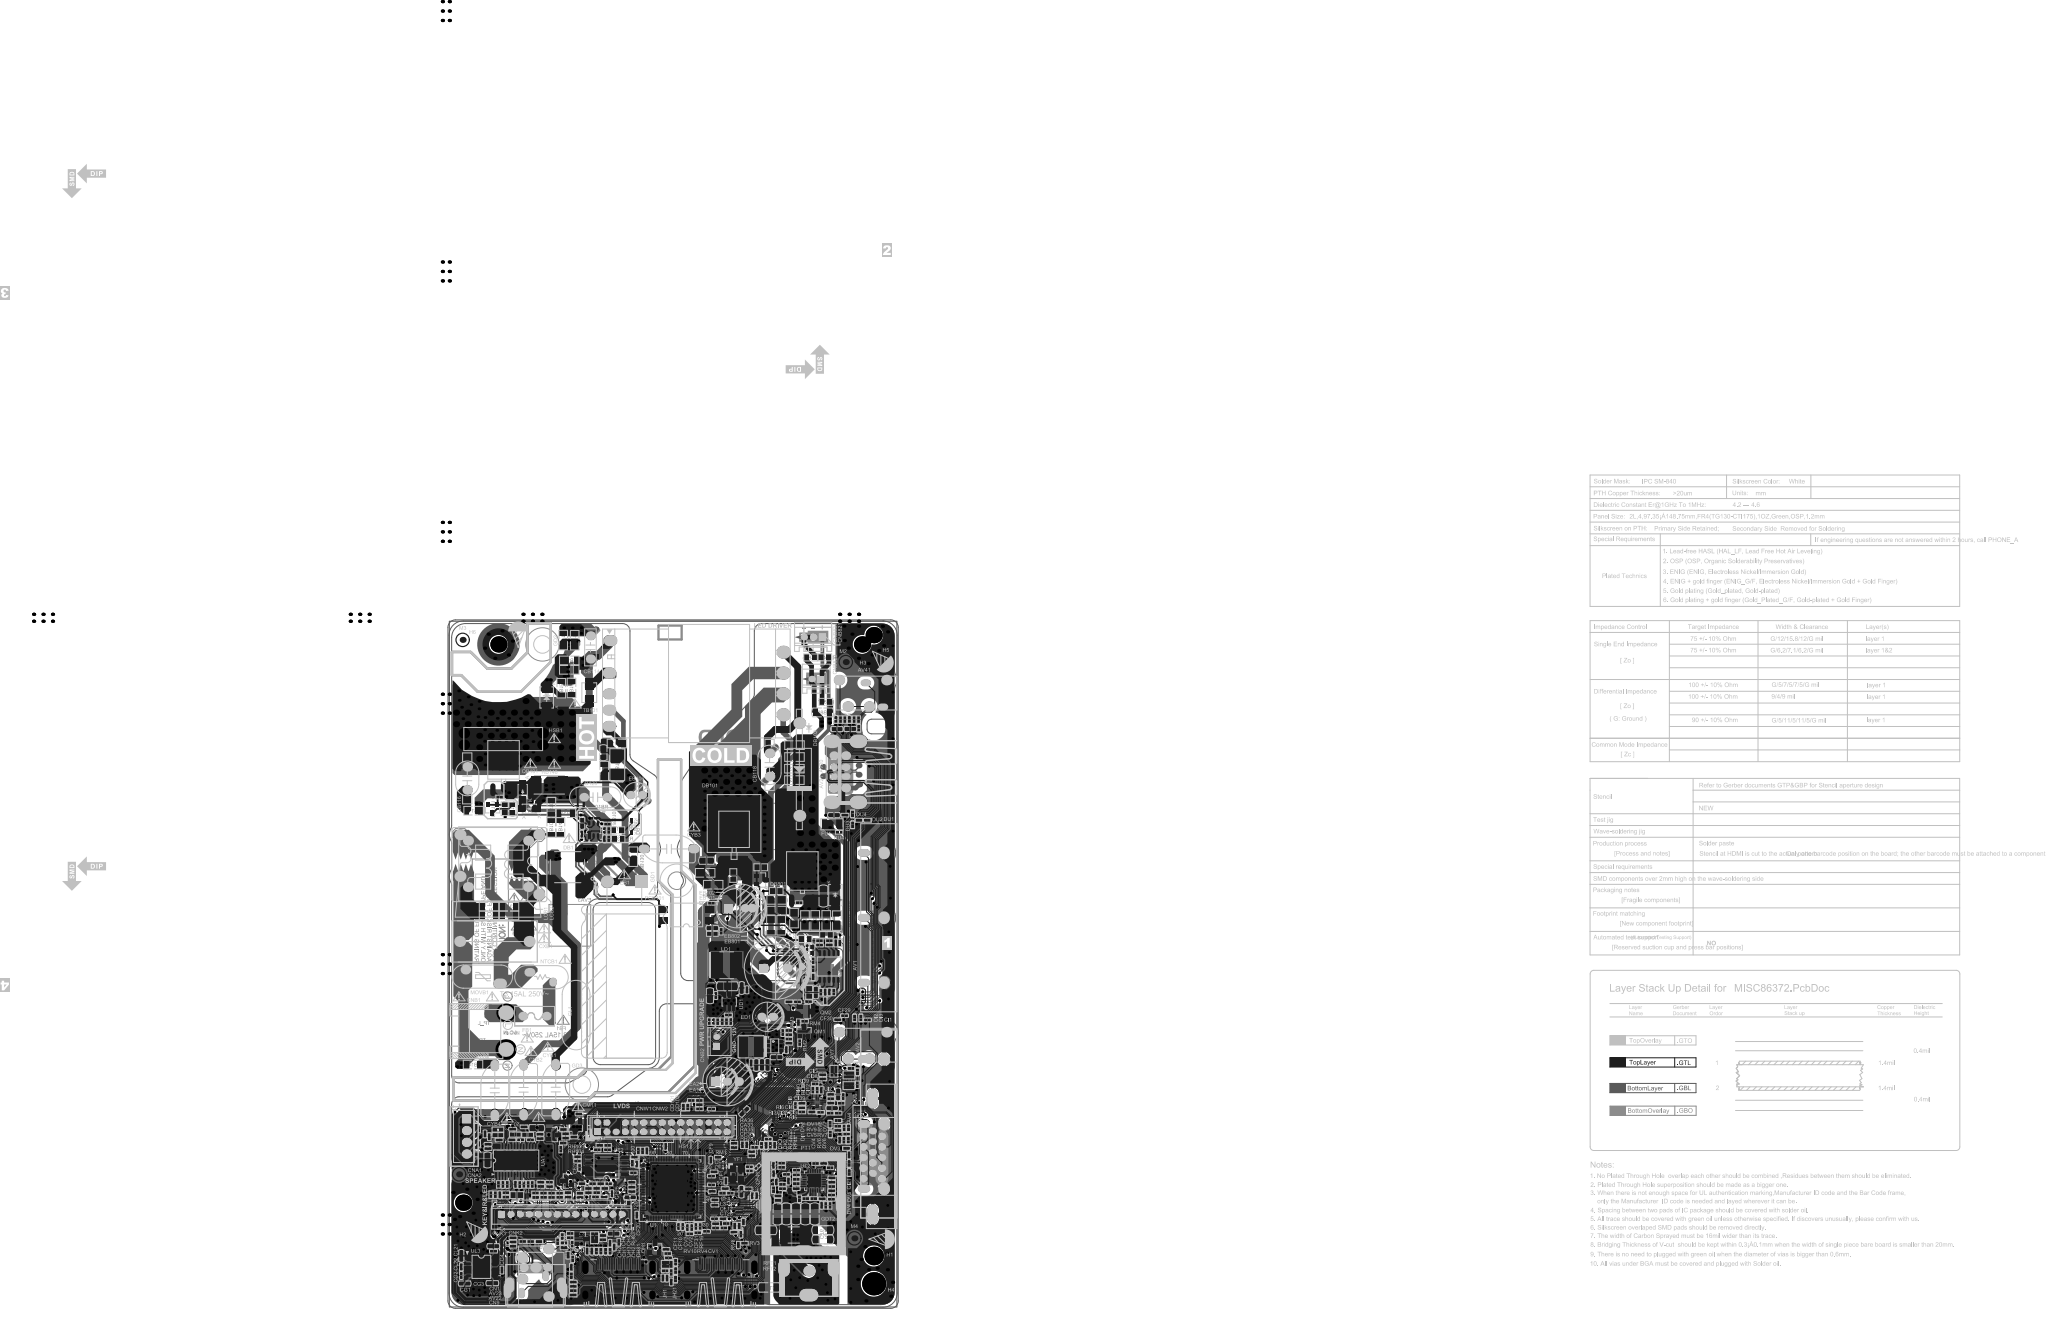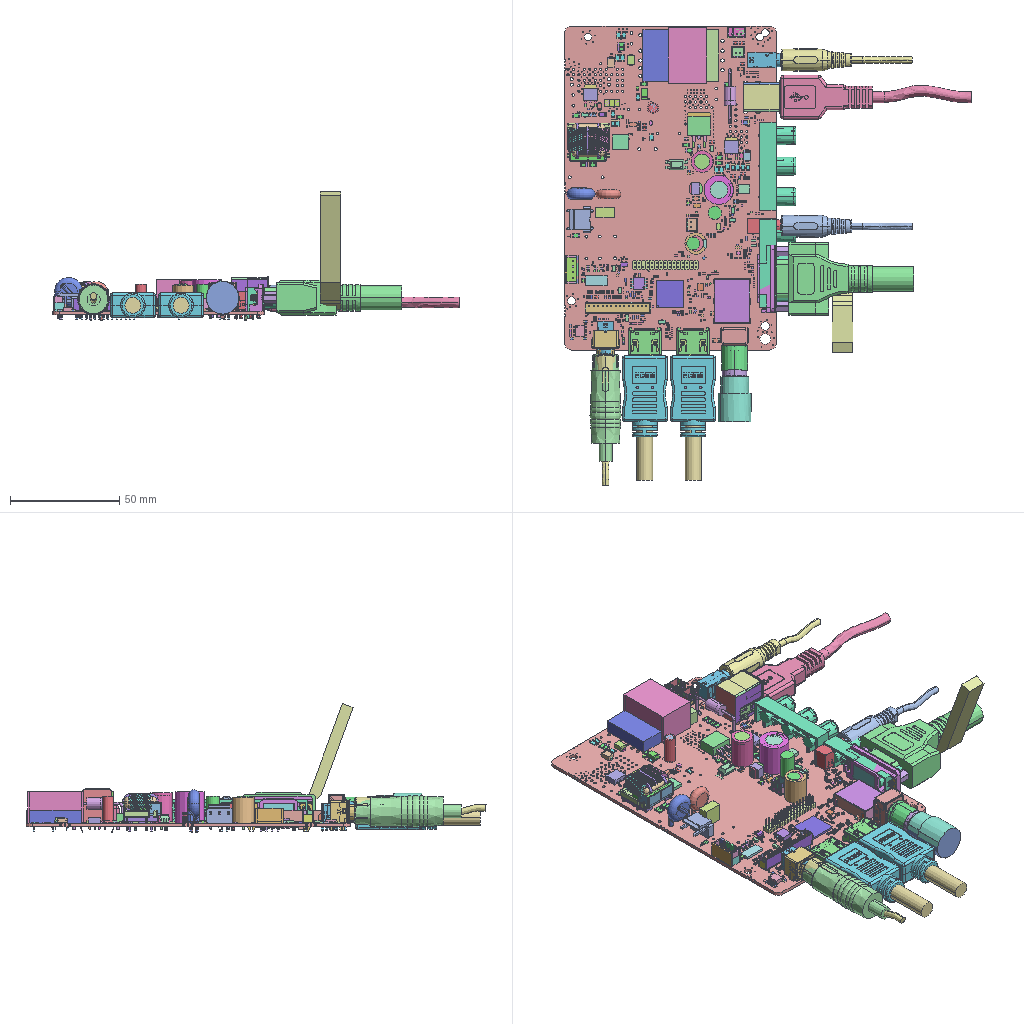Circuit board layout | Altium Designer | box 185.9 x 210.3 x 58.9 mm
Layer stack:
# Altium Designer layer stack of  (unit mm; dielectric type: 0 none, 1 core, 2 prepreg, 3 surface material)
index,name,kind,layer,copper_thickness_mm,dielectric_type,dielectric_thickness_mm,dielectric_material,dielectric_constant
0,TopPaste,other,,,,,,
1,TopOverlay,other,,,,,,
2,TopSolder,dielectric,,,3,0.0102,Solder Resist,3.5
3,TopLayer,copper,TopLayer,0.0356,,,,
4,Dielectric1,dielectric,,,1,1.5,FR-4,4.8
5,BottomLayer,copper,BottomLayer,0.0356,,,,
6,BottomSolder,dielectric,,,3,0.0102,Solder Resist,3.5
7,BottomOverlay,other,,,,,,
8,BottomPaste,other,,,,,,
# drill layer pairs: low layer,high layer
drill_pair,TopLayer,BottomLayer
Part placement, first 359 of 579 lines:
Designator,Comment,Layer,Footprint,Center-X(mm),Center-Y(mm),Rotation
DI6,NC/NC/AVLC18S02003,TopLayer,DIODE-S0402,-71.831,13.818,180
CO13,NC/1000pF-0402-X7R-¡À10%-50V,TopLayer,C0402,-71.831,12.802,180
CO12,NC/Ceramic capacitor,CAP MC,6.3V,0.47uF,¡À10%,X5R,0402,SMD,TP,TopLayer,C0402,-70.968,11.176,270
Manufacture_Info,Manufacture_Info,TopLayer,Manufacture_Info,-31.626,103.746,180
CT47,NC/Ceramic capacitor,CAP MC,1KV,4700pF,¡À10%,X7R,1206,SMD,TP,TopLayer,C1206,-28.27,16.56,360
CK3,Ceramic capacitor,CAP MC,50V,0.01uF,¡À10%,X7R,0402,SMD,TP,TopLayer,C0402,-63.17,23.749,180
RK13,33Kohm-0402-¡À5%-1/16W,TopLayer,R0402,-65.678,26.594,180
UF2,SPI FLASH chip,IC SPI FLASH,4MB,32Mb,SOIC8,SMD,W25Q32JVSSIQ,Winbond,TopLayer,SOIC8,-62.687,30.42,180
DV1,NC/AVLC18S02003,TopLayer,DIODE-S0402,-12.733,40.234,360
RT1,Ferrite bead,BEAD,300ohm,0402,800mA,SMD,TP,FCM1005KF-301T08,TopLayer,R0402,-35.941,24.566,180
RF9,NC/4K7ohm-0402-¡À5%-1/16W,TopLayer,R0402,-44.374,44.564,360
RF8,NC/4K7ohm-0402-¡À5%-1/16W,TopLayer,R0402,-42.647,44.564,180
EA2,NC/Aluminium electrolytic capacitor,CAP AL,16V,220uF,¡À20%,LD,KF,P,2.5mm,6.3¡Á11,DIP,TP,CapXon,TopLayer,EC(6.3*11)-V-2.5,-37.908,48.199,360
CNA2,NC/4PIN-2.54-D-H-G-latched-B,TopLayer,SIP4/2.5D-2,-92.877,36.793,270
CL4,NC/1uF-0402-X5R-¡À20%-6.3V,TopLayer,C0402,-26.01,26.988,90
CL3,10uF-0603-X5R-¡À20%-6.3V,TopLayer,C0603,-33.55,24.889,270
CI1,NC/10pF-0402-NPO-¡À5%-50V,TopLayer,C0402,-6.35,61.951,180
UART_TX,DM0,BottomLayer,TP,-25.349,49.047,90
RPI1,Resistor array,RES ARRAY,1/16W,4¡Á10Kohm,¡À5%,0402,SMD,TopLayer,RA0402,-13.589,50.876,180
DV8,NC/AVLC18S02003,TopLayer,DIODE-S0402,-9.881,51.486,180
DV9,NC/AVLC18S02003,TopLayer,DIODE-S0402,-8.509,50.749,270
RPV1,NC/Resistor array,RES ARRAY,1/16W,4¡Á10Kohm,¡À5%,0402,SMD,TopLayer,RA0402,-10.342,50.082,270
RF43,4K7ohm-0402-¡À5%-1/16W,TopLayer,R0402,-27.305,34.9,270
RF44,4K7ohm-0402-¡À5%-1/16W,TopLayer,R0402,-26.391,34.9,270
RU1,NC/0ohm-0402-PCB,TopLayer,R0402SC,-35.149,34.413,360
RU2,NC/0ohm-0402-PCB,TopLayer,R0402SC,-35.149,35.327,360
RU5,NC/0ohm-0402-PCB,TopLayer,R0402SC,-33.336,34.99,90
RI5,NC/0ohm-0402-¡À5%-1/16W,TopLayer,R0402,-16.471,41.992,180
CI3,NC/0.1uF-0402-X5R-¡À20%-16V,TopLayer,C0402,-16.471,41.993,360
CI4,NC/0.1uF-0402-X5R-¡À20%-16V,TopLayer,C0402,-20.496,42.996,360
CI6,0.1uF-0402-X5R-¡À20%-16V,TopLayer,C0402,-16.007,50.126,360
CV4,NC/30pF-0402-NPO-¡À5%-50V,TopLayer,C0402,-12.37,35.992,90
CV5,NC/30pF-0402-NPO-¡À5%-50V,TopLayer,C0402,-12.739,38.093,180
DV2,NC/AVLC18S02003,TopLayer,DIODE-S0402,-14.427,39.478,270
DV3,NC/AVLC18S02003,TopLayer,DIODE-S0402,-10.897,34.239,360
DV4,NC/AVLC18S02003,TopLayer,DIODE-S0402,-10.287,28.981,90
DV5,NC/AVLC18S02003,TopLayer,DIODE-S0402,-10.312,30.937,90
DV6,NC/AVLC18S02003,TopLayer,DIODE-S0402,-10.49,35.992,90
DV7,NC/AVLC18S02003,TopLayer,DIODE-S0402,-10.431,38.633,90
RF10,NC/100ohm-0402-¡À5%-1/16W,TopLayer,R0402,-42.639,43.649,360
RF11,NC/100ohm-0402-¡À5%-1/16W,TopLayer,R0402,-42.621,42.739,360
RM1,10Kohm-0402-¡À5%-1/16W,TopLayer,R0402,-38.608,32.309,180
RV6,NC/10Kohm-0402-¡À5%-1/16W,TopLayer,R0402,-11.43,35.992,90
RV7,NC/100ohm-0402-¡À5%-1/16W,TopLayer,R0402,-10.846,37.313,180
RV8,NC/10Kohm-0402-¡À5%-1/16W,TopLayer,R0402,-11.396,38.633,90
RV9,NC/100ohm-0402-¡À5%-1/16W,TopLayer,R0402,-12.751,39.011,180
RI6,NC/0ohm-0402-¡À5%-1/16W,TopLayer,R0402,-20.496,42.996,180
CA33,Ceramic capacitor,CAP MC,6.3V,0.47uF,¡À10%,X5R,0402,SMD,TP,TopLayer,C0402,-31.323,33.528,360
CI8,0.1uF-0402-X5R-¡À20%-16V,TopLayer,C0402,-21.895,43.51,90
CI9,NC/NC/10uF-0603-X5R-¡À20%-6.3V,TopLayer,C0603,-12.675,45.872,270
CI12,NC/Ceramic capacitor,CAP MC,6.3V,0.47uF,¡À10%,X5R,0402,SMD,TP,TopLayer,C0402,-16.298,46.805,90
CI35,NC/1000pF-0402-X7R-¡À10%-50V,TopLayer,C0402,-18.335,42.088,360
CI36,NC/0.1uF-0402-X5R-¡À20%-16V,TopLayer,C0402,-11.582,45.415,270
CI37,NC/Ceramic capacitor,CAP MC,6.3V,0.47uF,¡À10%,X5R,0402,SMD,TP,TopLayer,C0402,-14.275,45.868,360
CI38,NC/Ceramic capacitor,CAP MC,6.3V,0.47uF,¡À10%,X5R,0402,SMD,TP,TopLayer,C0402,-16.002,49.2,360
CI39,NC/Ceramic capacitor,CAP MC,6.3V,0.47uF,¡À10%,X5R,0402,SMD,TP,TopLayer,C0402,-20.502,43.94,180
CI40,NC/10uF-0603-X5R-¡À20%-6.3V,TopLayer,C0603,-13.97,42.901,180
CI41,NC/0.1uF-0402-X5R-¡À20%-16V,TopLayer,C0402,-14.275,43.993,180
RA35,47Kohm-0402-¡À5%-1/16W,TopLayer,R0402,-31.318,32.614,180
RA36,10Kohm-0402-¡À5%-1/16W,TopLayer,R0402,-30.709,34.442,360
RI3,NC/1Kohm-0402-¡À5%-1/16W,TopLayer,R0402,-20.498,42.088,360
RI4,0ohm-0402-¡À5%-1/16W,TopLayer,R0402,-8.534,47.955,90
RI37,NC/200Kohm-0402-¡À5%-1/16W,TopLayer,R0402,-14.275,44.929,360
RI38,NC/200Kohm-0402-¡À5%-1/16W,TopLayer,R0402,-17.212,46.804,90
RI39,NC/200Kohm-0402-¡À5%-1/16W,TopLayer,R0402,-17.653,48.133,180
RI40,NC/200Kohm-0402-¡À5%-1/16W,TopLayer,R0402,-18.127,46.804,90
RI42,NC/1Kohm-0402-¡À5%-1/16W,TopLayer,R0402,-12.675,41.834,360
RI43,NC/1Kohm-0402-¡À5%-1/16W,TopLayer,R0402,-12.04,43.967,360
RI48,NC/100ohm-0402-¡À5%-1/16W,TopLayer,R0402,-14.402,41.834,360
UI2,NC/AZAW2213F,TopLayer,QFN10/0.4,-17.206,44.208,270
CI21,NC/NC/10pF-0402-NPO-¡À5%-50V,TopLayer,C0402,-10.312,32.817,270
RU3,NC/0ohm-0402-PCB,TopLayer,R0402SC,-32.423,34.976,90
RA5,NC/?,TopLayer,GND,-32.31,21.262,180
RA4,NC/?,TopLayer,GND,-33.96,20.498,180
L6,0ohm-0402-¡À5%-1/16W,TopLayer,R0402,-14.427,30.041,180
CF40,Ceramic capacitor,CAP MC,50V,0.01uF,¡À10%,X7R,0402,SMD,TP,TopLayer,C0402,-30.099,30.201,225
UT2,Silicon RF tuner,IC Si Tuner,QFN24,SMD,R842,Rafael,TopLayer,QFN24/0.5-3,-17.882,27.254,90
RT8,100ohm-0402-¡À5%-1/16W,TopLayer,R0402,-17.551,30.963,180
RT6,1K8ohm-0402-¡À5%-1/16W,TopLayer,R0402,-14.05,25.988,180
RT5,0ohm-0402-¡À5%-1/16W,TopLayer,R0402,-24.867,31.039,180
RT4,0ohm-0402-¡À5%-1/16W,TopLayer,R0402,-24.867,30.124,180
RT3,22ohm-0402-¡À5%-1/16W,TopLayer,R0402,-14.431,21.924,90
RT2,22ohm-0402-¡À5%-1/16W,TopLayer,R0402,-15.345,21.924,90
LT10,NC/SDCL1005CR18JTDF(180nH-0402¡À5%-C),TopLayer,L0402,-24.707,26.474,180
LT9,Multilayer inductor,HF Inductor,270nH,¡À5%,0402,SMD,SDCL1005CR27JTDF,Sunlord,TopLayer,L0402,-21.717,27.564,180
LT8,Multilayer inductor,,HF Inductor,39nH,¡À5%,0402,SMD,SDCL1005C39NJTDF,Sunlord,TopLayer,L0402,-21.717,26.599,360
LT6,SDCL1005CR18JTDF(180nH-0402¡À5%-C),TopLayer,L0402,-17.933,23.368,180
LT5,GZ1005U102CTF(1000ohm-300mA),TopLayer,L0402,-19.66,23.368,180
LT4,GZ1005U102CTF(1000ohm-300mA),TopLayer,L0402,-21.031,23.343,270
LT3,NC/SDCL1005CR18JTDF(180nH-0402¡À5%-C),TopLayer,L0402,-26.619,25.299,90
LT2,NC/SDCL1005CR27JTDF(Sunlord),TopLayer,L0402,-25.654,23.012,180
CT27,0.1uF-0402-X5R-¡À20%-16V,TopLayer,C0402,-15.799,30.963,180
CT25,0.1uF-0402-X5R-¡À20%-16V,TopLayer,C0402,-14.021,27.864,360
CT24,6800pF-0402-X7R-¡À10%-50V,TopLayer,C0402,-14.072,25.07,180
CT23,330pF-0402-NPO-¡À5%-50V,TopLayer,C0402,-14.05,26.903,180
CT22,0.1uF-0402-X5R-¡À20%-16V,TopLayer,C0402,-14.117,24.154,360
CT21,0.1uF-0402-X5R-¡À20%-16V,TopLayer,C0402,-21.666,29.515,360
CT20,0.022uF-0402-X7R-¡À10%-16V,TopLayer,C0402,-23.829,28.6,180
CT19,0.022uF-0402-X7R-¡À10%-16V,TopLayer,C0402,-21.692,28.504,360
CT18,NC/1000pF-0402-X7R-¡À10%-50V,TopLayer,C0402,-23.393,27.178,270
CT17,0.1uF-0402-X5R-¡À20%-16V,TopLayer,C0402,-21.717,25.532,360
CT16,0.047uF-0402-X7R-¡À10%-16V,TopLayer,C0402,-16.129,23.343,360
CT15,0ohm-0402-¡À5%-1/16W,TopLayer,C0402,-24.706,25.535,360
CT14,NC/220pF-0402-NPO-¡À5%-50V,TopLayer,C0402,-25.654,23.952,180
CT10,NC/30pF-0402-NPO-¡À5%-50V,TopLayer,C0402,-26.645,30.582,90
CT8,NC/30pF-0402-NPO-¡À5%-50V,TopLayer,C0402,-26.619,28.727,90
CT7,Ceramic capacitor,CAP MC,50V,22pF,¡À5%,NPO,0402,SMD,TP,TopLayer,C0402,-14.117,23.239,180
CT6,Ceramic capacitor,CAP MC,50V,22pF,¡À5%,NPO,0402,SMD,TP,TopLayer,C0402,-16.259,21.95,90
DT1,KAV99,TopLayer,SO-23,-23.139,24.105,180
CF1,Ceramic capacitor,CAP MC,50V,18pF,¡À5%,NPO,0402,SMD,TP,TopLayer,C0402,-36.906,27.178,270
CF4,Ceramic capacitor,CAP MC,50V,18pF,¡À5%,NPO,0402,SMD,TP,TopLayer,C0402,-37.059,25.552,180
CF9,0.1uF-0402-X5R-¡À20%-16V,TopLayer,C0402,-40.174,31.689,270
CF10,0.1uF-0402-X5R-¡À20%-16V,TopLayer,C0402,-46.226,17.375,90
CF11,0.1uF-0402-X5R-¡À20%-16V,TopLayer,C0402,-47.14,17.375,270
CF12,0.1uF-0402-X5R-¡À20%-16V,TopLayer,C0402,-39.294,23.114,180
CF13,0.1uF-0402-X5R-¡À20%-16V,TopLayer,C0402,-39.115,17.975,180
CF14,0.1uF-0402-X5R-¡À20%-16V,TopLayer,C0402,-39.876,24.942,180
CF17,0.1uF-0402-X5R-¡À20%-16V,TopLayer,C0402,-40.005,26.34,180
CF19,0.1uF-0402-X5R-¡À20%-16V,TopLayer,C0402,-39.446,29.159,360
CF24,Ceramic capacitor,CAP MC,6.3V,2.2uF,¡À20%,X5R,0402,SMD,TP,TopLayer,C0402,-40.03,28.245,360
CF26,0.047uF-0402-X7R-¡À10%-16V,TopLayer,C0402,-39.116,17.044,360
CF27,NC/0.1uF-0402-X5R-¡À20%-16V,TopLayer,C0402,-37.484,19.043,180
CF28,1uF-0402-X5R-¡À20%-6.3V,TopLayer,C0402,-39.359,19.039,360
CF31,0.047uF-0402-X7R-¡À10%-16V,TopLayer,C0402,-43.383,17.373,270
CF38,NC/30pF-0402-NPO-¡À5%-50V,TopLayer,C0402,-31.833,30.251,360
CT11,0.1uF-0402-X5R-¡À20%-16V,TopLayer,C0402,-30.277,24.003,90
CT12,0.1uF-0402-X5R-¡À20%-16V,TopLayer,C0402,-31.191,24.003,90
CT26,0.022uF-0402-X7R-¡À10%-16V,TopLayer,C0402,-39.294,21.971,180
CV1,0.047uF-0402-X7R-¡À10%-16V,TopLayer,C0402,-41.097,16.307,180
CV2,0.047uF-0402-X7R-¡À10%-16V,TopLayer,C0402,-44.298,17.12,90
CV3,0.047uF-0402-X7R-¡À10%-16V,TopLayer,C0402,-45.215,17.12,90
L3,0ohm-0402-¡À5%-1/16W,TopLayer,L0402,-37.643,24.563,180
LF6,NC/?,TopLayer,GND,-37.998,19.66,180
RF12,68ohm-0402-¡À5%-1/16W,TopLayer,R0402,-37.338,17.043,360
RF16,68ohm-0402-¡À5%-1/16W,TopLayer,R0402,-42.469,17.374,90
RF24,1Kohm-0402-¡À5%-1/16W,TopLayer,R0402,-31.814,29.352,180
RV4,33ohm-0402-¡À5%-1/16W,TopLayer,R0402,-42.977,16.002,180
RV10,33ohm-0402-¡À5%-1/16W,TopLayer,R0402,-44.704,15.773,180
YF1,Passive crystal,SPXO,24MHz,¡À10ppm,12pF,SMD3225,SMD,2.3.3.240001234,MDH,TopLayer,XTAL-S-3,-34.519,28.677,270
DK2,NC/AVLC18S02003,TopLayer,DIODE-S0402,-28.245,34.9,270
DK3,NC/AVLC18S02003,TopLayer,DIODE-S0402,-29.21,34.9,270
CT1,NC/0.1uF-0402-X5R-¡À20%-16V,TopLayer,C0402,-27.737,36.22,180
RT7,10Kohm-0402-¡À5%-1/16W,TopLayer,R0402,-32.055,25.476,360
RK6,510ohm-0402-¡À1%-1/16W,TopLayer,R0402,-78.008,24.595,360
GDT2,NC/Gas discharge tube,GDT,700V,2000A,TP,4.5*3.2mm,SMD,4532-091-LF,Brightking,TopLayer,SMD4532-1-C1206,-16.002,15.57,270
GDT1,NC/Gas discharge tube,GDT,700V,2000A,TP,4.5*3.2mm,SMD,4532-091-LF,Brightking,TopLayer,SMD4532-1,-22.25,15.57,360
CT46,Thick-film resistor,RES,1/4W,0ohm,¡À5%,1206,SMD,TopLayer,C1206,-15.977,14.554,180
CT45,Thick-film resistor,RES,1/4W,0ohm,¡À5%,1206,SMD,TopLayer,C1206,-15.977,16.586,180
CT44,Thick-film resistor,RES,1/4W,0ohm,¡À5%,1206,SMD,TopLayer,C1206,-17.729,20.091,270
CT43,Thick-film resistor,RES,1/4W,0ohm,¡À5%,1206,SMD,TopLayer,C1206,-19.761,20.091,270
CT42,Thick-film resistor,RES,1/4W,0ohm,¡À5%,1206,SMD,TopLayer,C1206,-21.768,20.091,270
CT41,Thick-film resistor,RES,1/4W,0ohm,¡À5%,1206,SMD,TopLayer,C1206,-25.756,20.066,270
CT13,Ceramic capacitor,CAP MC,1KV,470pF,¡À5%,NPO,1206,SMD,TP,TopLayer,C1206,-23.851,20.091,90
RO12,NC/510ohm-0402-¡À1%-1/16W,TopLayer,R0402,-69.977,10.363,270
UA1,Audio amplifier,IC Audio AMP,Class D,2¡Á10W@13.0V@8ohm,HTSSOP-28,SMD,RDA3118E28B,RDA,TopLayer,SSOP28/0.65-5,-82.197,31.611,90
QM12,Field-effect transistor,PMOS,-4.3A,-30V,0.048ohm@ID=-3A@VGS=-4.5V,SOT-23-3L,NCE3407AY,NCEPOWER,TopLayer,SOT-23-1,-69.421,38.982,360
RA9,NC/47Kohm-0402-¡À5%-1/16W,TopLayer,R0402,-84.397,23.724,180
VCC_PANEL,TEST,BottomLayer,TP,-67.742,39.878,270
UART_RX,DM0,BottomLayer,TP,-27.686,49.276,90
TXD,,BottomLayer,TP,-62.56,22.631,180
RU4,0ohm-0402-¡À5%-1/16W,TopLayer,R0402,-12.464,102.457,180
RO22,75ohm-0402-¡À5%-1/16W,TopLayer,R0402,-55.804,33.68,270
RO21,Thick-film resistor,RES,1/16W,150ohm,¡À1%,0402,SMD,TopLayer,R0402,-54.89,33.674,270
RM15,NC/4K7ohm-0402-¡À5%-1/16W,TopLayer,R0402,-71.501,37.363,180
RM14,47Kohm-0402-¡À5%-1/16W,TopLayer,R0402,-71.501,36.452,360
RM12,10Kohm-0402-¡À5%-1/16W,TopLayer,R0402,-72.542,34.061,270
RK15,10Kohm-0402-¡À5%-1/16W,TopLayer,R0402,-66.573,24.648,360
RK14,510ohm-0402-¡À1%-1/16W,TopLayer,R0402,-64.795,24.666,360
RK12,4K7ohm-0402-¡À1%-1/16W,TopLayer,R0402,-76.246,23.658,360
RK11,2K2ohm-0402-¡À1%-1/16W,TopLayer,R0402,-74.534,23.641,360
RK10,1Kohm-0402-¡À5%-1/16W,TopLayer,R0402,-68.395,24.544,180
RK9,1K2ohm-0402-¡À1%-1/16W,TopLayer,R0402,-74.535,24.567,360
RK8,1Kohm-0402-¡À1%-1/16W,TopLayer,R0402,-72.791,24.559,360
RK7,680ohm-0402-¡À1%-1/16W,TopLayer,R0402,-72.782,23.663,360
RK5,22ohm-0402-¡À5%-1/16W,TopLayer,R0402,-70.993,24.669,360
RK4,1Kohm-0402-¡À5%-1/16W,TopLayer,R0402,-64.808,25.585,180
QM11,General transistor,Dynatron,NPN,0.2A,40V,30-300,SOT-23,MMBT3904(f¡Ý350MHz),BLUE ROCKET,TopLayer,SOT-23,-74.117,37.211,90
QK1,General transistor,Dynatron,NPN,0.2A,40V,30-300,SOT-23,MMBT3904(f¡Ý350MHz),BLUE ROCKET,TopLayer,SOT-23,-71.171,27.178,270
HS1,NC/Heatsink,6-series aluminium alloy,14.0¡Á14.0¡Á6.0mm,natural,XXWJ,TopLayer,HS(14*14*6),-582.797,-376.375,0
FU1,NC/NSMD110(1206-1.1A),TopLayer,FUSE1.1A-S,-13.994,104.165,180
DK1,NC/AVLC18S02003,TopLayer,DIODE-S0402,-78.01,23.648,360
CO31,NC/NC/33pF-0402-NPO-¡À5%-50V,TopLayer,C0402,-53.975,33.681,90
CO11,NC/1000pF-0402-X7R-¡À10%-50V,TopLayer,C0402,-70.257,8.56,90
CM12,0.022uF-0402-X7R-¡À10%-16V,TopLayer,C0402,-69.694,36.68,180
CM11,NC/0.1uF-0402-X5R-¡À20%-16V,TopLayer,C0402,-68.595,41.652,180
CL21,10uF-0603-X5R-¡À20%-6.3V,TopLayer,C0603,-94.018,11.032,90
CK5,NC/0.1uF-0402-X5R-¡À20%-16V,TopLayer,C0402,-65.056,23.752,360
CK4,NC/0.1uF-0402-X5R-¡À20%-16V,TopLayer,C0402,-68.37,23.63,180
+1.8V_DDR,TEST,BottomLayer,TP,-59.817,23.216,90
UL3,LDO regulator,IC LDO,1A,3.3V,12V,ESOP-8,SMD,LC1118CS8TR1833,Leadchip,TopLayer,SOP8/1.27-3,-89.689,8.66,360
RO33,NC/0ohm-0402-¡À5%-1/16W,TopLayer,R0402,-82.855,13.106,360
RO4,NC/0ohm-0402-¡À5%-1/16W,TopLayer,R0402,-79.045,14.118,180
RO3,NC/0ohm-0402-¡À5%-1/16W,TopLayer,R0402,-80.762,14.129,360
RO2,NC/0ohm-0402-¡À5%-1/16W,TopLayer,R0402,-73.228,14.072,90
DI9,NC/NC/SFI0402-240E-2R5PP-LF,TopLayer,DIODE-S0402,-77.241,14.101,180
CO33,330pF-0402-NPO-¡À5%-50V,TopLayer,C0402,-82.855,14.935,360
CO32,0.1uF-0402-X5R-¡À20%-16V,TopLayer,C0402,-82.855,14.021,180
CG4,1uF-0402-X5R-¡À20%-6.3V,TopLayer,C0402,-85.25,7.959,270
CG3,NC/10uF-0603-X5R-¡À20%-6.3V,TopLayer,C0603,-87.323,5.13,360
CG2,NC/Ceramic capacitor,CAP MC,6.3V,2.2uF,¡À20%,X5R,0402,SMD,TP,TopLayer,C0402,-94.027,6.802,270
CL24,1uF-0402-X5R-¡À20%-6.3V,TopLayer,C0402,-87.065,12.038,360
CL23,NC/10uF-0603-X5R-¡À20%-6.3V,TopLayer,C0603,-87.114,13.106,180
CL22,NC/Ceramic capacitor,CAP MC,6.3V,2.2uF,¡À20%,X5R,0402,SMD,TP,TopLayer,C0402,-94.018,8.64,270
CF16,0.1uF-0402-X5R-¡À20%-16V,TopLayer,C0402,-56.185,30.861,270
RK2,1Kohm-0402-¡À5%-1/16W,TopLayer,R0402,-64.668,33.925,360
CA5,0.22uF-0402-X5R-¡À10%-16V,TopLayer,C0402,-85.033,26.448,90
CA6,0.22uF-0402-X5R-¡À10%-16V,TopLayer,C0402,-84.075,26.448,90
CA7,1uF-0402-X5R-¡À20%-16V,TopLayer,C0402,-82.324,26.468,90
CA8,1uF-0402-X5R-¡À20%-16V,TopLayer,C0402,-81.417,26.406,90
CA9,1uF-0402-X5R-¡À20%-16V,TopLayer,C0402,-78.689,26.448,90
CA10,0.22uF-0402-X5R-¡À10%-16V,TopLayer,C0402,-76.864,26.92,180
RA1,4K7ohm-0402-¡À5%-1/16W,TopLayer,R0402,-87.641,24.236,270
RA2,4K7ohm-0402-¡À5%-1/16W,TopLayer,R0402,-86.001,26.459,270
RA3,1Kohm-0402-¡À5%-1/16W,TopLayer,R0402,-86.672,24.222,90
RA14,1Kohm-0402-¡À5%-1/16W,TopLayer,R0402,-76.849,26.01,360
CA3,3300pF-0402-X7R-¡À10%-50V,TopLayer,C0402,-85.714,24.197,90
CA4,3300pF-0402-X7R-¡À10%-50V,TopLayer,C0402,-74.939,25.984,180
CK1,NC/22pF-0402-NPO-¡À5%-50V,TopLayer,C0402,-62.439,33.941,360
RA8,NC/100Kohm-0402-¡À5%-1/16W,TopLayer,R0402,-84.397,24.638,180
RA10,10Kohm-0402-¡À1%-1/16W,TopLayer,R0402,-80.502,26.448,90
RA11,15Kohm-0402-¡À1%-1/16W,TopLayer,R0402,-79.588,26.448,90
CNK2,Connector socket,connect jack,14Pin,D2.0,D,Fool-proofing,Nature,L=2.8,DIP,W2011-14SVA-SN9-ENSY,XYDT,TopLayer,SIP14/2.0D-1,-72.365,19.99,360
CNK1,NC/Connector socket,connect jack,14Pin,D2.0,D,SNAP,Nature,L=2.8mm,DIP,AMA,TopLayer,SIP14/2.0D-5,-72.365,19.99,360
DI1,NC/AVLC18S02003,TopLayer,DIODE-S0402,-14.378,37.373,270
DI2,NC/AVLC18S02003,TopLayer,DIODE-S0402,-9.119,62.357,90
DI3,NC/AVLC18S02003,TopLayer,DIODE-S0402,-7.772,62.357,90
DM1,DM0,BottomLayer,TP,-8.251,114.876,180
DP1,DM0,BottomLayer,TP,-8.251,116.876,180
5V,DM0,BottomLayer,TP,-8.128,112.776,180
DU1,NC/TVS diode,DIO ESD,0.1pF,25V,0402,SMD,GESD1005H150CR10GPT,Sunlord,TopLayer,DIODE-S0402,-6.35,105.054,180
DU2,NC/TVS diode,DIO ESD,0.1pF,25V,0402,SMD,GESD1005H150CR10GPT,Sunlord,TopLayer,DIODE-S0402,-8.23,105.054,360
DU3,NC/TVS diode,DIO ESD,0.1pF,25V,0402,SMD,GESD1005H150CR10GPT,Sunlord,TopLayer,DIODE-S0402,-9.55,104.038,90
DU4,NC/TVS diode,DIO ESD,0.1pF,25V,0402,SMD,GESD1005H150CR10GPT,Sunlord,TopLayer,DIODE-S0402,-9.576,106.451,270
CU1,1uF-0402-X5R-¡À20%-6.3V,TopLayer,C0402,-11.197,106.147,360
CU2,NC/10uF-0603-X5R-¡À20%-6.3V,TopLayer,C0603,-13.578,106.153,180
PT1,Shield can,tinplate,natural,20.3¡Á16.3¡Á6mm,with sealed opening,LHD,TopLayer,SHIELD(16*20*6),-20.117,22.268,0
用于U1,NC/Glue, 0.1g, silicone,TopLayer,Heat-Shrinkable_Tube,-44.936,29.365,90
CN1,NC/RCA jack,RCA Jack,AV1,H,Yellow,CH5.5,Seal,DIP,AV38A-01S-5030,QS,TopLayer,AV1-H-4,-78,6.05,360
CH81,Ceramic capacitor,CAP MC,6.3V,0.47uF,¡À10%,X5R,0402,SMD,TP,TopLayer,C0402,-61.925,13.745,90
RH82,33Kohm-0402-¡À5%-1/16W,TopLayer,R0402,-70.536,15.861,360
RH81,22Kohm-0402-¡À5%-1/16W,TopLayer,R0402,-70.536,14.935,360
CNW1,NC/NC/Connector socket,connect jack,2¡Á15Pin/without pin6,D2.0,D,SNAP,Fool-proofing,Nature,L=2.6mm,DIP,CJ,TopLayer,SIP2*15/2.0D-11,-50.681,38.796,180
3V3_STB,TEST,BottomLayer,TP,-59.258,34.366,270
CD101,NC/NC?,TopLayer,DIODE-S0402,-46.096,43.12,90
CD102,NC/NC?,TopLayer,DIODE-S0402,-45.131,43.145,90
CF3,10uF-0603-X5R-¡À20%-6.3V,TopLayer,C0603,-57.614,23.628,360
CF5,10uF-0603-X5R-¡À20%-6.3V,TopLayer,C0603,-61.112,15.824,180
CF7,0.1uF-0402-X5R-¡À20%-16V,TopLayer,C0402,-49.911,34.671,270
CF8,0.1uF-0402-X5R-¡À20%-16V,TopLayer,C0402,-57.202,24.914,360
CF15,10uF-0603-X5R-¡À20%-6.3V,TopLayer,C0603,-32.918,42.164,225
CF18,0.1uF-0402-X5R-¡À20%-16V,TopLayer,C0402,-57.209,26.898,180
CF20,0.1uF-0402-X5R-¡À20%-16V,TopLayer,C0402,-56.138,19.813,90
CF21,Ceramic capacitor,CAP MC,6.3V,0.47uF,¡À10%,X5R,0402,SMD,TP,TopLayer,C0402,-57.201,25.832,180
CF25,Ceramic capacitor,CAP MC,6.3V,0.47uF,¡À10%,X5R,0402,SMD,TP,TopLayer,C0402,-61.493,24.435,90
CH101,NC/10pF-0402-NPO-¡À5%-50V,TopLayer,C0402,-48.692,5.385,270
CH102,NC/10pF-0402-NPO-¡À5%-50V,TopLayer,C0402,-49.604,6.223,90
CK2,NC/0.1uF-0402-X5R-¡À20%-16V,TopLayer,C0402,-71,23.688,360
CNW2,Gold pin,pin connector,2¡Á15Pin/without pin6,D,D2.0mm,L=2.6mm,DIP,H2030-30SVB-V06-J8SY,XYDT,TopLayer,SIP2*15/2.0D-2,-50.681,38.796,180
QM1,General transistor,Dynatron,NPN,0.2A,40V,30-300,SOT-23,MMBT3904(f¡Ý350MHz),BLUE ROCKET,TopLayer,SOT-23,-20.041,59.462,180
RK1,4K7ohm-0402-¡À5%-1/16W,TopLayer,R0402,-67.97,26.594,180
RF3,NC/4K7ohm-0402-¡À5%-1/16W,TopLayer,R0402,-56.865,28.931,180
RF13,4K7ohm-0402-¡À5%-1/16W,TopLayer,R0402,-62.433,34.87,360
RF23,4K7ohm-0402-¡À5%-1/16W,TopLayer,R0402,-57.099,31.029,90
RF29,4K7ohm-0402-¡À5%-1/16W,TopLayer,R0402,-56.642,32.36,180
RG61,NC/,TopLayer,R0402SC,-64.135,34.87,180
RH4,Resistor array,RES ARRAY,1/16W,4¡Á10Kohm,¡À5%,0402,SMD,TopLayer,RA0402,-65.253,14.935,360
RH5,33ohm-0402-¡À5%-1/16W,TopLayer,R0402,-63.43,15.418,360
RH6,33ohm-0402-¡À5%-1/16W,TopLayer,R0402,-63.449,14.495,360
RH25,33ohm-0402-¡À5%-1/16W,TopLayer,R0402,-50.038,7.798,180
RH26,33ohm-0402-¡À5%-1/16W,TopLayer,R0402,-48.717,7.442,270
RH83,100ohm-0402-¡À5%-1/16W,TopLayer,R0402,-60.02,13.938,270
RH102,Thick-film resistor,RES,1/16W,1.2Kohm,¡À1%,0402,SMD,TopLayer,R0402,-63.043,25.578,360
RH104,4K7ohm-0402-¡À5%-1/16W,TopLayer,R0402,-68.936,31.487,360
RH106,4K7ohm-0402-¡À5%-1/16W,TopLayer,R0402,-68.936,32.401,360
RK3,4K7ohm-0402-¡À1%-1/16W,TopLayer,R0402,-66.575,25.569,180
RXD,,BottomLayer,TP,-62.23,28.423,90
VDDC_CORE,TEST,BottomLayer,TP,-36.513,34.9,360
CF2,0.1uF-0402-X5R-¡À20%-16V,TopLayer,C0402,-68.504,30.115,270
RK16,15Kohm-0402-¡À1%-1/16W,TopLayer,R0402,-76.275,24.573,360
CG201,NC/0.1uF-0402-X5R-¡À20%-16V,TopLayer,C0402,-40.005,42.723,360
AV1,RCA jack,RCA Jack,AV3,H,Yellow¡¢White¡¢Red,CH5.5,D14,Seal,DIP,AV3-8.4-15C,JSL(MI material),TopLayer,AV3-H14-15,-4.925,84,90
CA1,10uF-0805-X5R-¡À20%-16V,TopLayer,C0805,-88.367,31.725,90
CA2,NC/10uF-0805-X5R-¡À20%-16V,TopLayer,C0805,-77.749,38.583,180
CA12,NC/0.1uF-0402-X5R-¡À20%-16V,TopLayer,C0402,-88.243,35.105,360
CA13,1000pF-0402-X7R-¡À10%-50V,TopLayer,C0402,-88.267,34.188,360
CA14,0.22uF-0402-X5R-¡À10%-16V,TopLayer,C0402,-85.852,36.043,360
CA15,0.22uF-0402-X5R-¡À10%-16V,TopLayer,C0402,-83.077,36.069,180
CA16,0.22uF-0402-X5R-¡À10%-16V,TopLayer,C0402,-81.208,36.086,360
CA17,0.22uF-0402-X5R-¡À10%-16V,TopLayer,C0402,-79.063,36.068,180
CA18,NC/0.1uF-0402-X5R-¡À20%-16V,TopLayer,C0402,-76.995,36.347,180
CA19,1000pF-0402-X7R-¡À10%-50V,TopLayer,C0402,-77.025,37.272,180
CA26,2200pF-0402-X7R-¡À10%-50V,TopLayer,C0402,-82.927,38.371,180
CA27,2200pF-0402-X7R-¡À10%-50V,TopLayer,C0402,-80.463,38.869,360
CA31,10uF-0603-X5R-¡À20%-6.3V,TopLayer,C0603,-12.954,124.714,180
CA32,10uF-0603-X5R-¡À20%-6.3V,TopLayer,C0603,-10.062,124.765,180
CD8,0.1uF-0402-X5R-¡À20%-16V,TopLayer,C0402,-24.638,59.233,90
CD10,NC/10uF-0603-X5R-¡À20%-6.3V,TopLayer,C0603,-27.911,52.248,270
CD12,NC/NC/3300pF-0402-X7R-¡À10%-50V,TopLayer,C0402,-23.297,56.911,360
CD13,NC/0.1uF-0402-X5R-¡À20%-16V,TopLayer,C0402,-31.453,52.654,270
CD14,10uF-0603-X5R-¡À20%-6.3V,TopLayer,C0603,-29.115,52.222,270
CD15,10uF-0603-X5R-¡À20%-6.3V,TopLayer,C0603,-30.341,52.206,270
CM1,0.1uF-0402-X5R-¡À20%-16V,TopLayer,C0402,-23.306,65.863,180
CM2,NC/0.1uF-0402-X5R-¡À20%-16V,TopLayer,C0402,-19.053,65.913,360
CM3,NC/0.022uF-0402-X7R-¡À10%-16V,TopLayer,C0402,-21.453,65.862,180
DM0,DM0,BottomLayer,TP,-15.925,114.556,180
DP0,DM0,BottomLayer,TP,-15.925,116.556,180
LD2,Power inductor,Power Inductor,2.2uH,¡À20%,2A,0.28¡Á1P,DR4.5¡Á3.2,SMD,PIO43-2R2MTP02,FH,TopLayer,L(4.5*3.5)-S,-31.453,56.185,360
QM2,Field-effect transistor,PMOS,-4.2A,-30V,0.052ohm@ID=-4.2A@VGS=-10V,SOT-23-3,AO3401,BLUE ROCKET,TopLayer,SOT-23-1,-19.751,63.762,90
RA25,10ohm-0805-¡À5%-1/8W,TopLayer,R0805,-82.019,24.13,180
RD9,Thick-film resistor,RES,1/16W,12Kohm,¡À1%,0402,SMD,TopLayer,R0402,-23.305,57.83,180
RM11,4K7ohm-0402-¡À5%-1/16W,TopLayer,R0402,-72.028,35.377,180
UD2,DC-DC converter,IC DCDC,Syn,1.2A,6.0V,1.5MHz,SOT23-5,SMD,TMI3408,TOLL,TopLayer,SOT-23-5,-26.365,56.343,270
EA1,Aluminium electrolytic capacitor,CAP AL,16V,470uF,¡À20%,KM,P,5.0mm,10¡Á12.5,DIP,TP,Samxon,TopLayer,EC(10*12)-V-5,-36.658,49.24,360
AI_V,AI_GRIPPER_V,TopLayer,AI_GRIPPER_V,30.243,27.653,90
AV4,RCA jack,RCA Jack,AV3,H,Green¡¢Blue¡¢Red,CH5.5,D14,Seal,DIP,AV3-8.4-15C,JSL,TopLayer,AV3-H14-15,-4.925,39.5,90
AV6,NC/WLHD-051A,TopLayer,DB15-HF-1,-5.247,32.5,90
AV7,NC/Earphone jack,Earphone Jack,H,¦µ3.5,CH7.0,Black,Seal,DIP,PJ-373,JSL,TopLayer,PHONE-HD-41,-7.375,56.45,90
AV20,USB jack,USB Jack,H,Single,flange,DIP,WLUS-050F USB,WLCO,TopLayer,USB1-HD-2,-9.655,115.5,90
AV21,NC/USB jack,USB Jack,H,Double,Black,flange,DIP,WLUS-074B,WLCO,TopLayer,USB2-HD-1,-11.15,115.5,90
AV22,RCA jack,RCA Jack,AV1,H,Orange,CH5.5,Seal,DIP,RCA-143A-EP-07,CS,TopLayer,AV1-H-4,-78,6.05,0
AV23,NC/Optical jack,OPTICAL,H,DIP,182500191,VAST,TopLayer,OPTICAL-HD-3,-78,6.6,0
AV41,Earphone jack,Earphone Jack,H,¦µ3.5,CH7.0,Black,switch,Seal,DIP,PJ-373A,JSL,TopLayer,PHONE-HD-42,-7.375,132.4,90
BA1,Ferrite bead,BEAD,600ohm,0603,2A,SMD,TP,EPZ1608E601-2R0TF,Sunlord,TopLayer,L0603,-86.12,37.073,180
BA2,Ferrite bead,BEAD,600ohm,0603,2A,SMD,TP,EPZ1608E601-2R0TF,Sunlord,TopLayer,L0603,-86.114,38.295,180
BA3,Ferrite bead,BEAD,600ohm,0603,2A,SMD,TP,EPZ1608E601-2R0TF,Sunlord,TopLayer,L0603,-82.372,37.211,180
BA4,Ferrite bead,BEAD,600ohm,0603,2A,SMD,TP,EPZ1608E601-2R0TF,Sunlord,TopLayer,L0603,-79.705,37.16,180
CA24,2200pF-0402-X7R-¡À10%-50V,TopLayer,C0402,-87.979,36.751,270
CA25,2200pF-0402-X7R-¡À10%-50V,TopLayer,C0402,-88.9,37.338,270
CD16,10uF-0603-X5R-¡À20%-6.3V,TopLayer,C0603,-25.96,53.904,360
CD17,NC/0.1uF-0402-X5R-¡À20%-16V,TopLayer,C0402,-23.849,55.525,270
CH1,NC/0.1uF-0402-X5R-¡À20%-16V,TopLayer,C0402,-65.862,12.044,90
CH2,NC/0.1uF-0402-X5R-¡À20%-16V,TopLayer,C0402,-66.861,12.049,90
CH3,NC/Ceramic capacitor,CAP MC,50V,22pF,¡À5%,NPO,0402,SMD,TP,TopLayer,C0402,-50.507,6.244,270
CH4,NC/Ceramic capacitor,CAP MC,50V,22pF,¡À5%,NPO,0402,SMD,TP,TopLayer,C0402,-61.006,12.928,270
CH21,NC/0.1uF-0402-X5R-¡À20%-16V,TopLayer,C0402,-49.313,10.59,360
CH22,NC/0.1uF-0402-X5R-¡À20%-16V,TopLayer,C0402,-49.828,12.421,180
CN9,NC/Earphone jack,Earphone Jack,H,¦µ3.5,CH7.0,Black,switch,Seal,DIP,PJ-373A,JSL,TopLayer,PHONE-HD-42,-78.1,7.375,0
CNA1,Connector socket,connect jack,4Pin,D2.5,D,Nature,L=2.8mm,DIP,W2411-04SVA-ENSY,XYDT,TopLayer,SIP4/2.54D-1,-92.877,36.793,270
CO14,NC/1000pF-0402-X7R-¡À10%-50V,TopLayer,C0402,-69.887,2.577,360
CO15,NC/Ceramic capacitor,CAP MC,6.3V,0.47uF,¡À10%,X5R,0402,SMD,TP,TopLayer,C0402,-69.85,4.431,360
CO16,NC/1000pF-0402-X7R-¡À10%-50V,TopLayer,C0402,-69.85,5.371,180
DA31,NC/NC?,TopLayer,DIODE-S0402,-10.251,126.771,90
DA32,NC/NC?,TopLayer,DIODE-S0402,-13.157,126.771,90
DA33,NC/NC?,TopLayer,DIODE-S0402,-8.23,124.894,90
DBS0,DOLBY,BottomLayer,DOLBY-SILK,-582.797,-376.375,180
DH1,Ceramic capacitor,CAP MC,50V,22pF,¡À5%,NPO,0402,SMD,TP,TopLayer,DIODE-S0402,-61.906,12.04,270
DH2,NC/SFI0402-240E-2R5PP-LF,TopLayer,DIODE-S0402,-63.881,12.065,270
DH3,NC/SFI0402-240E-2R5PP-LF,TopLayer,DIODE-S0402,-64.861,12.065,270
DH21,Ceramic capacitor,CAP MC,50V,22pF,¡À5%,NPO,0402,SMD,TP,TopLayer,DIODE-S0402,-47.777,6.002,90
DH22,NC/SFI0402-240E-2R5PP-LF,TopLayer,DIODE-S0402,-47.752,7.828,90
DH23,NC/SFI0402-240E-2R5PP-LF,TopLayer,DIODE-S0402,-47.752,9.677,270
DH81,NC/SFI0402-240E-2R5PP-LF,TopLayer,DIODE-S0402,-62.865,12.04,270
DI8,NC/NC/SFI0402-240E-2R5PP-LF,TopLayer,DIODE-S0402,-70.275,6.768,270
JH1,HDMI jack,HDMI Jack,H,SMD,161031041(hull-SPCC ),VAST,TopLayer,HDMI-HS-1,-59.999,5.719,0
JH21,HDMI jack,HDMI Jack,H,SMD,161031041(hull-SPCC ),VAST,TopLayer,HDMI-HS-1,-37.999,5.719,0
LOUT+,DM0,BottomLayer,TP,-90.627,33.096,180
LOUT-,DM0,BottomLayer,TP,-90.627,35.636,180
QH1,General transistor,Dynatron,NPN,0.2A,40V,30-300,SOT-23,MMBT3904(f¡Ý350MHz),BLUE ROCKET,TopLayer,SOT-23,-68.072,14.58,90
Pad and via stacks, first 72 of 273 lines:
# Altium Designer via and pad stacks of  (unit mm). Each distinct definition once, with the count of objects using it.
# via: kind,start_layer,end_layer,hole_mm,diameter_mm,mode(0 simple;1 top-mid-bottom;2 full stack),diameter_per_layer,count,example_net
# pad: kind,layer,hole_mm,hole_type(0 round;1 square;2 slot),plating,top_size,top_shape(1 round;2 rect;3 octagon;9 rounded rect),mid_size,bottom_size,mode,footprint,size_per_layer,count,example
pad,TopOverlay,0,0,plated,2.7x1.7,1,2.7x1.7,2.7x1.7,0,AV3-H14-15,,9,AV2.0
pad,TopOverlay,0,0,plated,2.8x2.5,1,2.8x2.5,2.8x2.5,0,AV3-H14-15,,9,AV2.0
pad,TopOverlay,0,0,plated,2.1x2.1,1,2.1x2.1,2.1x2.1,0,CAP8.5*5-V-5,,2,CB118.0
pad,TopOverlay,0,0,plated,2.1x4.1,1,2.1x4.1,2.1x4.1,0,SHIELD(16*20*6),,4,PT1.0
pad,TopOverlay,0,0,plated,1.8x1.8,1,1.8x1.8,1.8x1.8,0,EC(6.3*11)-V-2.5,,4,ED1.5
pad,TopOverlay,0,0,plated,1.9x1.9,1,1.9x1.9,1.9x1.9,0,EC(10*12)-V-5,,1,EA1.0
pad,TopOverlay,0,0,plated,1.9x1.9,2,1.9x1.9,1.9x1.9,0,EC(10*12)-V-5,,1,EA1.0
pad,TopOverlay,0,0,plated,1.3x1.3,1,1.3x1.3,1.3x1.3,0,SIP2*15/2.0D-2,,28,CNW2.0
pad,TopOverlay,0,0,plated,1.3x1.3,2,1.3x1.3,1.3x1.3,0,SIP2*15/2.0D-2,,1,CNW2.0
pad,TopOverlay,0,0,plated,1.3x1.3,1,1.3x1.3,1.3x1.3,0,SIP2*15/2.0D-11,,28,CNW1.374
pad,TopOverlay,0,0,plated,1.3x1.3,2,1.3x1.3,1.3x1.3,0,SIP2*15/2.0D-11,,1,CNW1.372
pad,TopOverlay,0,0,plated,1.3x1.3,2,1.3x1.3,1.3x1.3,0,SIP14/2.0D-1,,1,CNK2.0
pad,TopOverlay,0,0,plated,1.3x1.3,1,1.3x1.3,1.3x1.3,0,SIP14/2.0D-1,,13,CNK2.0
pad,TopOverlay,0,0,plated,2.2x2.2,1,2.2x2.2,2.2x2.2,0,AV1-H-4,,2,CN1.2
pad,TopOverlay,0,0,plated,3.4x1.6,1,3.4x1.6,3.4x1.6,0,AV1-H-4,,4,CN1.3
pad,TopOverlay,0,0,plated,2.3x1.5,1,2.3x1.5,2.3x1.5,0,PHONE-HD-42,,4,CN9.8
pad,TopOverlay,0,0,plated,2.3x2.3,1,2.3x2.3,2.3x2.3,0,PHONE-HD-42,,8,CN9.0
pad,TopOverlay,0,0,plated,1.778x1.778,1,1.778x1.778,1.778x1.778,0,OPTICAL-HD-3,,3,AV23.0
pad,TopOverlay,0,0,plated,2x3.4,1,2x3.4,2x3.4,0,OPTICAL-HD-3,,2,AV23.0
pad,TopOverlay,0,0,plated,1.905x1.905,1,1.905x1.905,1.905x1.905,0,SIP4/2.54D-1,,3,CNA1.0
pad,TopOverlay,0,0,plated,1.905x1.905,2,1.905x1.905,1.905x1.905,0,SIP4/2.54D-1,,1,CNA1.0
pad,TopOverlay,0,0,plated,1.905x1.905,1,1.905x1.905,1.905x1.905,0,SIP4/2.5D-2,,3,CNA2.0
pad,TopOverlay,0,0,plated,1.905x1.905,2,1.905x1.905,1.905x1.905,0,SIP4/2.5D-2,,1,CNA2.0
pad,TopOverlay,0,0,plated,1.3x1.3,2,1.3x1.3,1.3x1.3,0,SIP14/2.0D-5,,1,CNK1.0
pad,TopOverlay,0,0,plated,1.3x1.3,1,1.3x1.3,1.3x1.3,0,SIP14/2.0D-5,,13,CNK1.0
pad,TopOverlay,0,0,plated,2.4x2.4,1,2.4x2.4,2.4x2.4,0,ANT-IEC14.5-H-4,,1,RFT1.0
pad,TopOverlay,0,0,unplated,2.5x3.8,1,2.5x3.8,2.5x3.8,0,ANT-IEC14.5-H-4,,2,RFT1.0
pad,TopOverlay,0,0,unplated,2.7x4.1,1,2.7x4.1,2.7x4.1,0,ANT-IEC14.5-H-4,,1,RFT1.0
pad,TopOverlay,0,0,plated,2.3x2.3,1,2.3x2.3,2.3x2.3,0,T-13.2\u00A1\u00C112.4\u00A1\u00C17.7-F14.5,,1,RFT2.0
pad,TopOverlay,0,0,unplated,2.5x3.8,1,2.5x3.8,2.5x3.8,0,T-13.2\u00A1\u00C112.4\u00A1\u00C17.7-F14.5,,2,RFT2.0
pad,TopOverlay,0,0,unplated,2.7x4.1,1,2.7x4.1,2.7x4.1,0,T-13.2\u00A1\u00C112.4\u00A1\u00C17.7-F14.5,,1,RFT2.0
pad,TopOverlay,0,0,plated,2.4x4.4,1,2.4x4.4,2.4x4.4,0,DB15-HF-1,,2,AV6.0
pad,TopOverlay,0,0,plated,1.5x1.5,1,1.5x1.5,1.5x1.5,0,DB15-HF-1,,15,AV6.44
pad,TopOverlay,0,0,plated,2.3x2.3,1,2.3x2.3,2.3x2.3,0,PHONE-HD-41,,4,AV7.5
pad,TopOverlay,0,0,plated,1.4x1.4,1,1.4x1.4,1.4x1.4,0,USB2-HD-1,,4,AV21.0
pad,TopOverlay,0,0,plated,1.85x1.85,1,1.85x1.85,1.85x1.85,0,USB2-HD-1,,4,AV21.0
pad,TopOverlay,0,0,plated,2.9x3.7,1,2.9x3.7,2.9x3.7,0,USB2-HD-1,,4,AV21.0
pad,TopOverlay,0,0,plated,2.1x1.7,1,2.1x1.7,2.1x1.7,0,USB1-HD-2,,2,AV20.0
pad,TopOverlay,0,0,plated,2.7x3.9,1,2.7x3.9,2.7x3.9,0,USB1-HD-2,,2,AV20.0
pad,TopOverlay,0,0,plated,1.4x2.1,1,1.4x2.1,1.4x2.1,0,USB1-HD-2,,2,AV20.1
pad,TopOverlay,0,0,unplated,2.4x3,1,2.4x3,2.4x3,0,T/EQ2414*10,,5,TB101.0
pad,TopOverlay,0,0,unplated,2.9x2.9,1,2.9x2.9,2.9x2.9,0,T/EQ2414*10,,4,TB101.0
pad,TopOverlay,0,0,plated,2.4x1.9,1,2.4x1.9,2.4x1.9,0,NTC(10*5)-V5,,1,NTCB1.3
pad,TopOverlay,0,0,plated,1.7x2,1,1.7x2,1.7x2,0,NTC(10*5)-V5,,1,NTCB1.2
pad,TopOverlay,0,0,plated,2.1x2.1,1,2.1x2.1,2.1x2.1,0,VR(13*5)-V-7.5,,1,MOVB1.2
pad,TopOverlay,0,0,plated,2.2x3,1,2.2x3,2.2x3,0,VR(13*5)-V-7.5,,1,MOVB1.2
pad,TopOverlay,0,0,plated,2.4x2.4,1,2.4x2.4,2.4x2.4,0,L/LC4/20.5*16-H-17*9(12.9),,4,LCB2.8
pad,TopOverlay,0,0,plated,2.2x2.2,1,2.2x2.2,2.2x2.2,0,L/UU10.5/10*13-2,,4,LCB1.4
pad,TopOverlay,0,0,plated,1.8x1.8,2,1.8x1.8,1.8x1.8,0,EC(8*11)-V-3.5,,1,EB102.1
pad,TopOverlay,0,0,plated,1.8x1.8,1,1.8x1.8,1.8x1.8,0,EC(8*11)-V-3.5,,1,EB102.1
pad,TopOverlay,0,0,plated,1.9x1.9,2,1.9x1.9,1.9x1.9,0,EC(10*12.5)-V-5,,2,EB101.1
pad,TopOverlay,0,0,plated,1.9x1.9,1,1.9x1.9,1.9x1.9,0,EC(10*12.5)-V-5,,2,EB101.1
pad,TopOverlay,0,0,plated,2.7x2.7,1,2.7x2.7,2.7x2.7,0,EC(18*31.5)-H-7.5,,1,EB1.2
pad,TopOverlay,0,0,plated,2.7x2.7,2,2.7x2.7,2.7x2.7,0,EC(18*31.5)-H-7.5,,1,EB1.2
pad,TopOverlay,0,0,plated,2.6x2.6,1,2.6x2.6,2.6x2.6,0,D3-H-20,,2,DB102.0
pad,TopOverlay,0,0,plated,1.9x2.55,1,1.9x2.55,1.9x2.55,0,CAP13*5-V-10-1,,8,CYB4.61
pad,TopOverlay,0,0,plated,2.4x2.4,1,2.4x2.4,2.4x2.4,0,CAP18*8.5-V-15,,2,CXB1.77
pad,TopOverlay,0,0,plated,1.4x1.4,1,1.4x1.4,1.4x1.4,0,SIP3/2.0D-CP,,2,CNB831.0
pad,TopOverlay,0,0,plated,1.4x1.4,2,1.4x1.4,1.4x1.4,0,SIP3/2.0D-CP,,1,CNB831.0
pad,TopOverlay,0,0,plated,1.4x1.4,1,1.4x1.4,1.4x1.4,0,SIP2/2.0D-CP,,2,CNB822.0
pad,TopOverlay,0,0,plated,1.4x1.4,2,1.4x1.4,1.4x1.4,0,SIP2/2.0D-CP,,2,CNB822.0
pad,TopOverlay,0,0,plated,1.3x1.3,1,1.3x1.3,1.3x1.3,0,SIP2/2.0D-1,,1,CNB2.0
pad,TopOverlay,0,0,plated,1.3x1.3,2,1.3x1.3,1.3x1.3,0,SIP2/2.0D-1,,1,CNB2.0
pad,TopOverlay,0,0,plated,3.2x3.2,1,3.2x3.2,3.2x3.2,0,CON2-H7.92,,2,CNB1.110
pad,TopOverlay,0,0,plated,2x2,1,2x2,2x2,0,CAP8*2.5-V-5,,2,CB114.1
pad,TopOverlay,0,0,unplated,2.1x2.1,1,2.1x2.1,2.1x2.1,0,CAP7.5*5-V-5-1,,2,CB116.0
pad,TopOverlay,0,0,plated,1.9x1.9,1,1.9x1.9,1.9x1.9,0,CAP10*4.5-V-5,,2,CB120.41
pad,TopOverlay,0,0,plated,1.9x1.9,1,1.9x1.9,1.9x1.9,0,FUSE8.5*4-V-5(T3.15AL 250V~),,2,FB1.5
pad,TopOverlay,0,0,plated,1.9x1.9,1,1.9x1.9,1.9x1.9,0,EC(13*13)-V-5,,2,EB802.2
Copper pours:
name,layer,net,type(0 solid;1 hatched;2 none)
12mil,BottomLayer,GND1,0
gnd,BottomLayer,GND,0
6.2,BottomLayer,GND,0
fgnd,BottomLayer,RFGND,0
gnd,BottomLayer,GND,0
5,TopLayer,GND,0
12mil,TopLayer,D_QB801,0
6.2,TopLayer,GND,0
6.2,TopLayer,GND,0
6.2,TopLayer,GND,0
12,TopLayer,VDDC_CORE,0
12mil,TopLayer,,0
12mil,TopLayer,GND1,0
fgnd,TopLayer,RFGND,0
5,TopLayer,GND,0
gnd,TopLayer,GND,0
5,TopLayer,GND,0
Design rules, without the lines most boards share, first 24 of 33 lines:
# Altium Designer design rules of  (exported by Altium Designer, unit mm)
# columns: name | kind | enabled | priority | scope1 | scope2 | descriptor | typed fields (field=value)
NetAntennae | 56 | enabled | 1 | Not (HasFootprint('ANT-7') or HasFootprint('ANT-BLUECORE')) | All | Net Antennae (Tolerance=1.016mm) (Not (HasFootprint('ANT-7') or HasFootprint('ANT-BLUECORE'))) |
Hole2Hole | 52 | disabled | 1 | All | All | Hole To Hole Clearance (Gap=0.457mm) (Disabled)(All),(All) | gap=0.4572
DiffPairsRouting | 51 | enabled | 4 | All | All | Differential Pairs Uncoupled Length using the Gap Constraints (Min=0.254mm) (Max=0.254mm) (Prefered=0.254mm)  and Width Constraints (Min=0.381mm) (Max=0.381mm) (Prefered=0.381mm) (All) |
Height | 50 | enabled | 1 | All | All | Height Constraint (Min=0mm) (Max=25.4mm) (Prefered=12.7mm) (All) | min_height=0 max_height=25.4
TestPointUsage | 44 | enabled | 1 | All | All | Fabrication Testpoint Usage (Valid =One Required, Allow multiple per net=No) (All) |
Testpoint | 43 | enabled | 1 | All | All | Fabrication Testpoint Style (Under Component=Yes) (All) |
HoleSize_VIA | 42 | disabled | 1 | ISVIA | All | Hole Size Constraint (Min=0.2mm) (Max=0.6mm) (Disabled)(ISVIA) |
PermittedLayers | 26 | enabled | 1 | All | All | Permitted Layers - (Top Layer, Bottom Layer) (All) |
SMDToCorner | 23 | disabled | 1 | All | All | SMD To Corner (Distance=0.102mm) (Disabled)(All) |
MinimumAnnularRing | 19 | enabled | 1 | All | All | Minimum Annular Ring (Minimum=0.1mm) (All) |
ViasUnderSMD | 17 | enabled | 1 | All | All | Vias Under SMD Constraint (Allowed=Not Allowed) (All) |
PasteMaskExpansion | 14 | enabled | 1 | All | All | Paste Mask Expansion (Expansion =0mm) (All) | expansion=0
0.25_0.1 | 11 | disabled | 6 | All | All | Routing Via (MinHoleWidth=0.1mm) (MaxHoleWidth=0.1mm) (PreferredHoleWidth=0.1mm) (MinWidth=0.25mm) (MaxWidth=0.25mm) (PreferedWidth=0.25mm) (Disabled)(All) | via_min_hole=0.1 via_max_hole=0.1 via_preferred_diameter=0.25 via_preferred_hole=0.1
0.4_0.2 | 11 | disabled | 5 | All | All | Routing Via (MinHoleWidth=0.2mm) (MaxHoleWidth=0.2mm) (PreferredHoleWidth=0.2mm) (MinWidth=0.4mm) (MaxWidth=0.4mm) (PreferedWidth=0.4mm) (Disabled)(All) | via_min_hole=0.2 via_max_hole=0.2 via_preferred_diameter=0.4 via_preferred_hole=0.2
0.45_0.25 | 11 | disabled | 4 | All | All | Routing Via (MinHoleWidth=0.25mm) (MaxHoleWidth=0.25mm) (PreferredHoleWidth=0.25mm) (MinWidth=0.45mm) (MaxWidth=0.45mm) (PreferedWidth=0.45mm) (Disabled)(All) | via_min_hole=0.25 via_max_hole=0.25 via_preferred_diameter=0.45 via_preferred_hole=0.25
0.5_0.3 | 11 | disabled | 3 | All | All | Routing Via (MinHoleWidth=0.3mm) (MaxHoleWidth=0.3mm) (PreferredHoleWidth=0.3mm) (MinWidth=0.5mm) (MaxWidth=0.5mm) (PreferedWidth=0.5mm) (Disabled)(All) | via_min_hole=0.3 via_max_hole=0.3 via_preferred_diameter=0.5 via_preferred_hole=0.3
0.8_0.5 | 11 | disabled | 2 | All | All | Routing Via (MinHoleWidth=0.5mm) (MaxHoleWidth=0.5mm) (PreferredHoleWidth=0.5mm) (MinWidth=0.8mm) (MaxWidth=0.8mm) (PreferedWidth=0.8mm) (Disabled)(All) | via_min_hole=0.5 via_max_hole=0.5 via_preferred_diameter=0.8 via_preferred_hole=0.5
0.6_0.4 | 11 | enabled | 1 | All | All | Routing Via (MinHoleWidth=0.4mm) (MaxHoleWidth=0.4mm) (PreferredHoleWidth=0.4mm) (MinWidth=0.6mm) (MaxWidth=0.6mm) (PreferedWidth=0.6mm) (All) | via_min_hole=0.4 via_max_hole=0.4 via_preferred_diameter=0.6 via_preferred_hole=0.4
RoutingCorners | 10 | enabled | 1 | All | All | Routing Corners (Style=45-Degree) (Min Setback=2.54mm) (Max Setback=2.54mm) (All) |
DiffPair_HDMI_MatchedLengths | 4 | enabled | 3 | InDifferentialPairClass('HDMI') | All | Matched Lengths(Tolerance=2.54mm) (InDifferentialPairClass('HDMI')) |
DiffPair_LVDS_MatchedLengths | 4 | enabled | 2 | InDifferentialPairClass('LVDS') | All | Matched Lengths(Tolerance=2.54mm) (InDifferentialPairClass('LVDS')) |
DiffPair_USB_MatchedLengths | 4 | enabled | 1 | InDifferentialPairClass('USB') | All | Matched Lengths(Tolerance=2.54mm) (InDifferentialPairClass('USB')) |